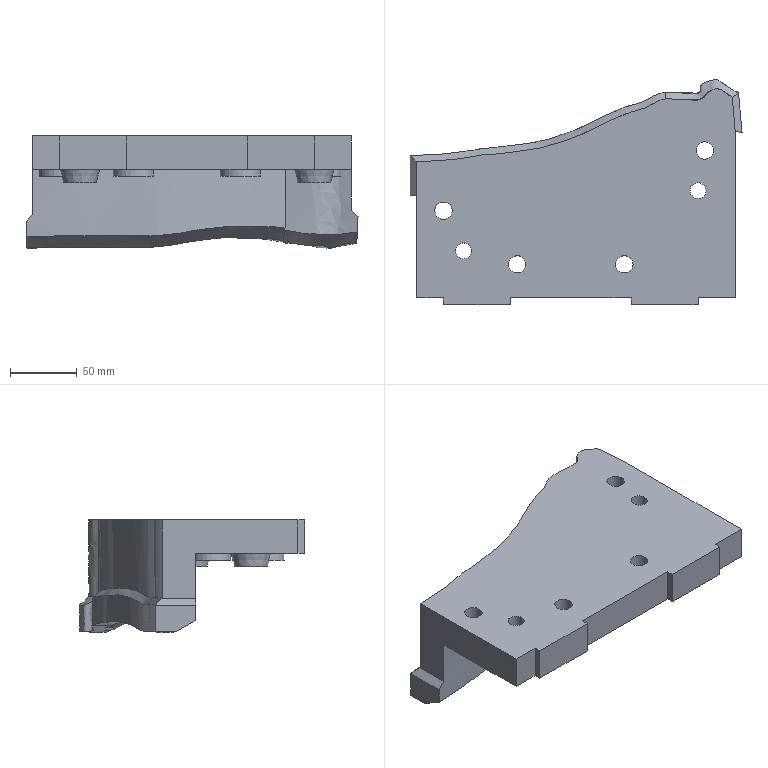Part | NX | features solid 2 | 1 solid | 56 faces | box 247.778 x 168.145 x 83.704 mm | volume 1113284 mm3 | plane 30 | spline 12 | cylinder 12 | cone 2 | commonest cylinder face diameters 13 x6 30 x4 12 x2